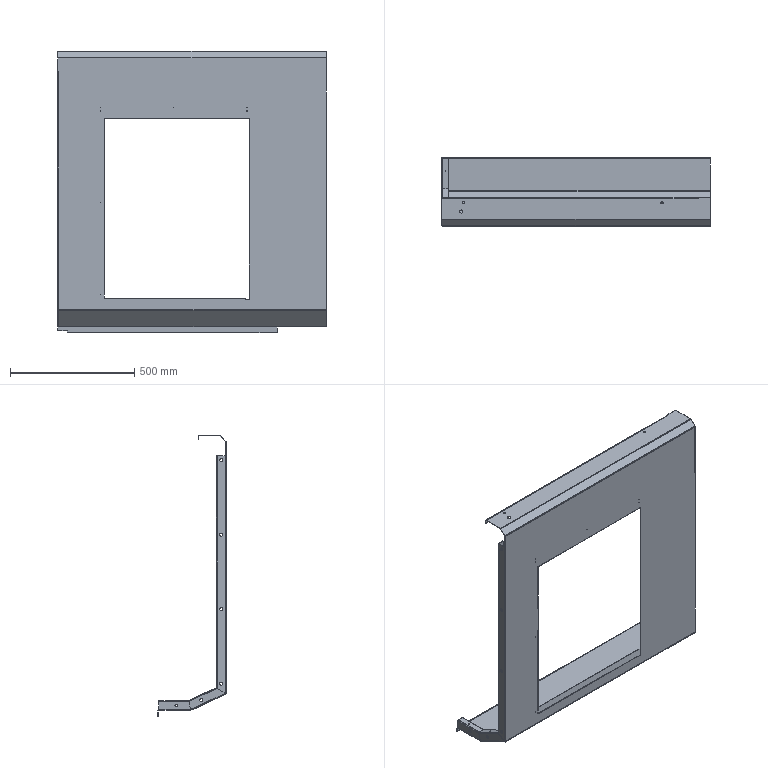Part | NX | features solid 2 | 1 solid | 145 faces | box 1083 x 275 x 1133 mm | volume 2454101 mm3 | cylinder 69 | plane 68 | spline 8 | commonest cylinder face diameters 1 x15 3.459 x12 4 x12 8 x12 12 x12 9.2 x4